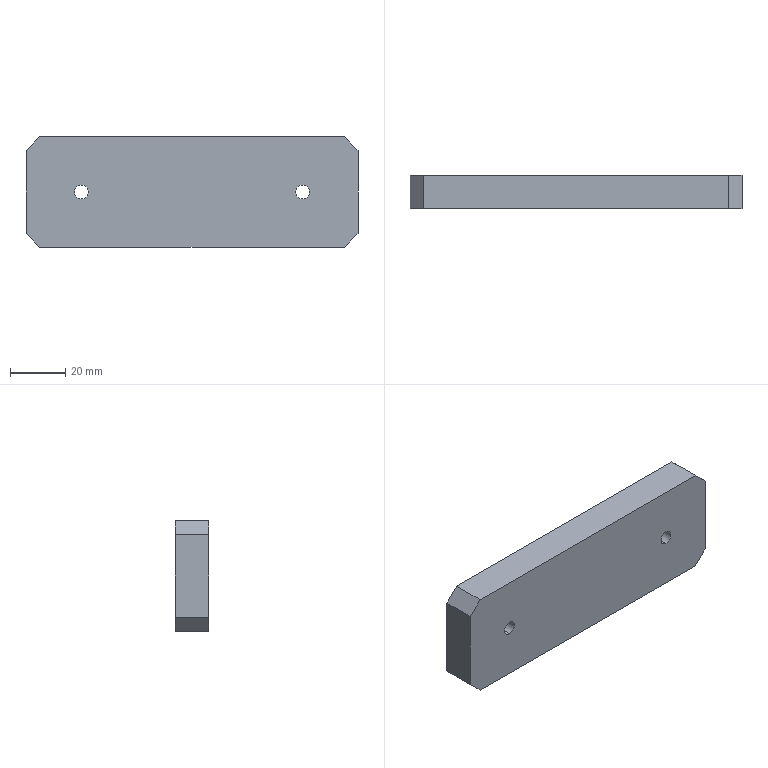Part | SolidWorks | features Chamfer 1, Extrusion 1, HoleWzd 1 | 1 solid | 14 faces | box 120 x 12 x 40 mm | volume 56529 mm3 | plane 10 | cylinder 4 | commonest cylinder face diameters 5 x4
STEP:
#1=CARTESIAN_POINT('',(-40.,-6.,-2.5));
#2=VERTEX_POINT('',#1);
#3=CARTESIAN_POINT('',(-40.,-6.,2.5));
#4=VERTEX_POINT('',#3);
#5=CARTESIAN_POINT('',(-40.,-6.,0.));
#6=DIRECTION('',(0.,1.,0.));
#7=DIRECTION('',(0.,0.,1.));
#8=AXIS2_PLACEMENT_3D('',#5,#6,#7);
#9=CIRCLE('',#8,2.5);
#10=EDGE_CURVE('',#2,#4,#9,.T.);
#11=ORIENTED_EDGE('',*,*,#10,.F.);
#12=CARTESIAN_POINT('',(-40.,6.,-2.5));
#13=VERTEX_POINT('',#12);
#14=CARTESIAN_POINT('',(-40.,6.,-2.5));
#15=DIRECTION('',(0.,1.,0.));
#16=VECTOR('',#15,1000.);
#17=LINE('',#14,#16);
#18=EDGE_CURVE('',#2,#13,#17,.T.);
#19=ORIENTED_EDGE('',*,*,#18,.T.);
#20=CARTESIAN_POINT('',(-40.,6.,2.5));
#21=VERTEX_POINT('',#20);
#22=CARTESIAN_POINT('',(-40.,6.,0.));
#23=DIRECTION('',(0.,1.,0.));
#24=DIRECTION('',(0.,0.,1.));
#25=AXIS2_PLACEMENT_3D('',#22,#23,#24);
#26=CIRCLE('',#25,2.5);
#27=EDGE_CURVE('',#13,#21,#26,.T.);
#28=ORIENTED_EDGE('',*,*,#27,.T.);
#29=CARTESIAN_POINT('',(-40.,6.,2.5));
#30=DIRECTION('',(0.,1.,0.));
#31=VECTOR('',#30,1000.);
#32=LINE('',#29,#31);
#33=EDGE_CURVE('',#4,#21,#32,.T.);
#34=ORIENTED_EDGE('',*,*,#33,.F.);
#35=EDGE_LOOP('',(#11,#19,#28,#34));
#36=FACE_OUTER_BOUND('',#35,.T.);
#37=CARTESIAN_POINT('',(-40.,6.,0.));
#38=DIRECTION('',(0.,1.,0.));
#39=DIRECTION('',(0.,0.,1.));
#40=AXIS2_PLACEMENT_3D('',#37,#38,#39);
#41=CYLINDRICAL_SURFACE('',#40,2.5);
#42=ADVANCED_FACE('',(#36),#41,.F.);
#43=CARTESIAN_POINT('',(40.,-6.,-2.5));
#44=VERTEX_POINT('',#43);
#45=CARTESIAN_POINT('',(40.,-6.,2.5));
#46=VERTEX_POINT('',#45);
#47=CARTESIAN_POINT('',(40.,-6.,0.));
#48=DIRECTION('',(0.,1.,0.));
#49=DIRECTION('',(0.,0.,1.));
#50=AXIS2_PLACEMENT_3D('',#47,#48,#49);
#51=CIRCLE('',#50,2.5);
#52=EDGE_CURVE('',#44,#46,#51,.T.);
#53=ORIENTED_EDGE('',*,*,#52,.F.);
#54=CARTESIAN_POINT('',(40.,6.,-2.5));
#55=VERTEX_POINT('',#54);
#56=CARTESIAN_POINT('',(40.,6.,-2.5));
#57=DIRECTION('',(0.,1.,0.));
#58=VECTOR('',#57,1000.);
#59=LINE('',#56,#58);
#60=EDGE_CURVE('',#44,#55,#59,.T.);
#61=ORIENTED_EDGE('',*,*,#60,.T.);
#62=CARTESIAN_POINT('',(40.,6.,2.5));
#63=VERTEX_POINT('',#62);
#64=CARTESIAN_POINT('',(40.,6.,0.));
#65=DIRECTION('',(0.,1.,0.));
#66=DIRECTION('',(0.,0.,1.));
#67=AXIS2_PLACEMENT_3D('',#64,#65,#66);
#68=CIRCLE('',#67,2.5);
#69=EDGE_CURVE('',#55,#63,#68,.T.);
#70=ORIENTED_EDGE('',*,*,#69,.T.);
#71=CARTESIAN_POINT('',(40.,6.,2.5));
#72=DIRECTION('',(0.,1.,0.));
#73=VECTOR('',#72,1000.);
#74=LINE('',#71,#73);
#75=EDGE_CURVE('',#46,#63,#74,.T.);
#76=ORIENTED_EDGE('',*,*,#75,.F.);
#77=EDGE_LOOP('',(#53,#61,#70,#76));
#78=FACE_OUTER_BOUND('',#77,.T.);
#79=CARTESIAN_POINT('',(40.,6.,0.));
#80=DIRECTION('',(0.,1.,0.));
#81=DIRECTION('',(0.,0.,1.));
#82=AXIS2_PLACEMENT_3D('',#79,#80,#81);
#83=CYLINDRICAL_SURFACE('',#82,2.5);
#84=ADVANCED_FACE('',(#78),#83,.F.);
#85=CARTESIAN_POINT('',(-60.,-6.,-15.));
#86=VERTEX_POINT('',#85);
#87=CARTESIAN_POINT('',(-60.,-6.,15.));
#88=VERTEX_POINT('',#87);
#89=CARTESIAN_POINT('',(-60.,-6.,-20.));
#90=DIRECTION('',(0.,0.,1.));
#91=VECTOR('',#90,1000.);
#92=LINE('',#89,#91);
#93=EDGE_CURVE('',#86,#88,#92,.T.);
#94=ORIENTED_EDGE('',*,*,#93,.T.);
#95=CARTESIAN_POINT('',(-60.,6.,15.));
#96=VERTEX_POINT('',#95);
#97=CARTESIAN_POINT('',(-60.,6.,15.));
#98=DIRECTION('',(0.,1.,0.));
#99=VECTOR('',#98,1000.);
#100=LINE('',#97,#99);
#101=EDGE_CURVE('',#88,#96,#100,.T.);
#102=ORIENTED_EDGE('',*,*,#101,.T.);
#103=CARTESIAN_POINT('',(-60.,6.,-15.));
#104=VERTEX_POINT('',#103);
#105=CARTESIAN_POINT('',(-60.,6.,-20.));
#106=DIRECTION('',(0.,0.,1.));
#107=VECTOR('',#106,1000.);
#108=LINE('',#105,#107);
#109=EDGE_CURVE('',#104,#96,#108,.T.);
#110=ORIENTED_EDGE('',*,*,#109,.F.);
#111=CARTESIAN_POINT('',(-60.,6.,-15.));
#112=DIRECTION('',(0.,-1.,0.));
#113=VECTOR('',#112,1000.);
#114=LINE('',#111,#113);
#115=EDGE_CURVE('',#104,#86,#114,.T.);
#116=ORIENTED_EDGE('',*,*,#115,.T.);
#117=EDGE_LOOP('',(#94,#102,#110,#116));
#118=FACE_OUTER_BOUND('',#117,.T.);
#119=CARTESIAN_POINT('',(-60.,6.,-20.));
#120=DIRECTION('',(1.,0.,0.));
#121=DIRECTION('',(0.,0.,-1.));
#122=AXIS2_PLACEMENT_3D('',#119,#120,#121);
#123=PLANE('',#122);
#124=ADVANCED_FACE('',(#118),#123,.F.);
#125=CARTESIAN_POINT('',(-55.,-6.,20.));
#126=VERTEX_POINT('',#125);
#127=CARTESIAN_POINT('',(55.,-6.,20.));
#128=VERTEX_POINT('',#127);
#129=CARTESIAN_POINT('',(-60.,-6.,20.));
#130=DIRECTION('',(1.,0.,0.));
#131=VECTOR('',#130,1000.);
#132=LINE('',#129,#131);
#133=EDGE_CURVE('',#126,#128,#132,.T.);
#134=ORIENTED_EDGE('',*,*,#133,.T.);
#135=CARTESIAN_POINT('',(55.,6.,20.));
#136=VERTEX_POINT('',#135);
#137=CARTESIAN_POINT('',(55.,6.,20.));
#138=DIRECTION('',(0.,1.,0.));
#139=VECTOR('',#138,1000.);
#140=LINE('',#137,#139);
#141=EDGE_CURVE('',#128,#136,#140,.T.);
#142=ORIENTED_EDGE('',*,*,#141,.T.);
#143=CARTESIAN_POINT('',(-55.,6.,20.));
#144=VERTEX_POINT('',#143);
#145=CARTESIAN_POINT('',(-60.,6.,20.));
#146=DIRECTION('',(1.,0.,0.));
#147=VECTOR('',#146,1000.);
#148=LINE('',#145,#147);
#149=EDGE_CURVE('',#144,#136,#148,.T.);
#150=ORIENTED_EDGE('',*,*,#149,.F.);
#151=CARTESIAN_POINT('',(-55.,6.,20.));
#152=DIRECTION('',(0.,-1.,0.));
#153=VECTOR('',#152,1000.);
#154=LINE('',#151,#153);
#155=EDGE_CURVE('',#144,#126,#154,.T.);
#156=ORIENTED_EDGE('',*,*,#155,.T.);
#157=EDGE_LOOP('',(#134,#142,#150,#156));
#158=FACE_OUTER_BOUND('',#157,.T.);
#159=CARTESIAN_POINT('',(-60.,6.,20.));
#160=DIRECTION('',(0.,0.,-1.));
#161=DIRECTION('',(-1.,0.,0.));
#162=AXIS2_PLACEMENT_3D('',#159,#160,#161);
#163=PLANE('',#162);
#164=ADVANCED_FACE('',(#158),#163,.F.);
#165=CARTESIAN_POINT('',(60.,6.,15.));
#166=VERTEX_POINT('',#165);
#167=CARTESIAN_POINT('',(60.,6.,-15.));
#168=VERTEX_POINT('',#167);
#169=CARTESIAN_POINT('',(60.,6.,-20.));
#170=DIRECTION('',(0.,0.,-1.));
#171=VECTOR('',#170,1000.);
#172=LINE('',#169,#171);
#173=EDGE_CURVE('',#166,#168,#172,.T.);
#174=ORIENTED_EDGE('',*,*,#173,.F.);
#175=CARTESIAN_POINT('',(60.,-6.,15.));
#176=VERTEX_POINT('',#175);
#177=CARTESIAN_POINT('',(60.,6.,15.));
#178=DIRECTION('',(0.,-1.,0.));
#179=VECTOR('',#178,1000.);
#180=LINE('',#177,#179);
#181=EDGE_CURVE('',#166,#176,#180,.T.);
#182=ORIENTED_EDGE('',*,*,#181,.T.);
#183=CARTESIAN_POINT('',(60.,-6.,-15.));
#184=VERTEX_POINT('',#183);
#185=CARTESIAN_POINT('',(60.,-6.,-20.));
#186=DIRECTION('',(0.,0.,-1.));
#187=VECTOR('',#186,1000.);
#188=LINE('',#185,#187);
#189=EDGE_CURVE('',#176,#184,#188,.T.);
#190=ORIENTED_EDGE('',*,*,#189,.T.);
#191=CARTESIAN_POINT('',(60.,6.,-15.));
#192=DIRECTION('',(0.,1.,0.));
#193=VECTOR('',#192,1000.);
#194=LINE('',#191,#193);
#195=EDGE_CURVE('',#184,#168,#194,.T.);
#196=ORIENTED_EDGE('',*,*,#195,.T.);
#197=EDGE_LOOP('',(#174,#182,#190,#196));
#198=FACE_OUTER_BOUND('',#197,.T.);
#199=CARTESIAN_POINT('',(60.,6.,-20.));
#200=DIRECTION('',(-1.,0.,0.));
#201=DIRECTION('',(0.,0.,1.));
#202=AXIS2_PLACEMENT_3D('',#199,#200,#201);
#203=PLANE('',#202);
#204=ADVANCED_FACE('',(#198),#203,.F.);
#205=CARTESIAN_POINT('',(55.,-6.,-20.));
#206=VERTEX_POINT('',#205);
#207=CARTESIAN_POINT('',(-55.,-6.,-20.));
#208=VERTEX_POINT('',#207);
#209=CARTESIAN_POINT('',(-60.,-6.,-20.));
#210=DIRECTION('',(-1.,0.,0.));
#211=VECTOR('',#210,1000.);
#212=LINE('',#209,#211);
#213=EDGE_CURVE('',#206,#208,#212,.T.);
#214=ORIENTED_EDGE('',*,*,#213,.T.);
#215=CARTESIAN_POINT('',(-55.,6.,-20.));
#216=VERTEX_POINT('',#215);
#217=CARTESIAN_POINT('',(-55.,6.,-20.));
#218=DIRECTION('',(0.,1.,0.));
#219=VECTOR('',#218,1000.);
#220=LINE('',#217,#219);
#221=EDGE_CURVE('',#208,#216,#220,.T.);
#222=ORIENTED_EDGE('',*,*,#221,.T.);
#223=CARTESIAN_POINT('',(55.,6.,-20.));
#224=VERTEX_POINT('',#223);
#225=CARTESIAN_POINT('',(-60.,6.,-20.));
#226=DIRECTION('',(-1.,0.,0.));
#227=VECTOR('',#226,1000.);
#228=LINE('',#225,#227);
#229=EDGE_CURVE('',#224,#216,#228,.T.);
#230=ORIENTED_EDGE('',*,*,#229,.F.);
#231=CARTESIAN_POINT('',(55.,6.,-20.));
#232=DIRECTION('',(0.,-1.,0.));
#233=VECTOR('',#232,1000.);
#234=LINE('',#231,#233);
#235=EDGE_CURVE('',#224,#206,#234,.T.);
#236=ORIENTED_EDGE('',*,*,#235,.T.);
#237=EDGE_LOOP('',(#214,#222,#230,#236));
#238=FACE_OUTER_BOUND('',#237,.T.);
#239=CARTESIAN_POINT('',(-60.,6.,-20.));
#240=DIRECTION('',(0.,0.,1.));
#241=DIRECTION('',(1.,0.,0.));
#242=AXIS2_PLACEMENT_3D('',#239,#240,#241);
#243=PLANE('',#242);
#244=ADVANCED_FACE('',(#238),#243,.F.);
#245=CARTESIAN_POINT('',(-40.,6.,0.));
#246=DIRECTION('',(0.,1.,0.));
#247=DIRECTION('',(0.,0.,1.));
#248=AXIS2_PLACEMENT_3D('',#245,#246,#247);
#249=CIRCLE('',#248,2.5);
#250=EDGE_CURVE('',#21,#13,#249,.T.);
#251=ORIENTED_EDGE('',*,*,#250,.F.);
#252=ORIENTED_EDGE('',*,*,#27,.F.);
#253=EDGE_LOOP('',(#251,#252));
#254=FACE_BOUND('',#253,.T.);
#255=CARTESIAN_POINT('',(40.,6.,0.));
#256=DIRECTION('',(0.,1.,0.));
#257=DIRECTION('',(0.,0.,1.));
#258=AXIS2_PLACEMENT_3D('',#255,#256,#257);
#259=CIRCLE('',#258,2.5);
#260=EDGE_CURVE('',#63,#55,#259,.T.);
#261=ORIENTED_EDGE('',*,*,#260,.F.);
#262=ORIENTED_EDGE('',*,*,#69,.F.);
#263=EDGE_LOOP('',(#261,#262));
#264=FACE_BOUND('',#263,.T.);
#265=ORIENTED_EDGE('',*,*,#149,.T.);
#266=CARTESIAN_POINT('',(-2.5,6.,77.5));
#267=DIRECTION('',(0.7071,0.,-0.7071));
#268=VECTOR('',#267,1000.);
#269=LINE('',#266,#268);
#270=EDGE_CURVE('',#136,#166,#269,.T.);
#271=ORIENTED_EDGE('',*,*,#270,.T.);
#272=ORIENTED_EDGE('',*,*,#173,.T.);
#273=CARTESIAN_POINT('',(17.5,6.,-57.5));
#274=DIRECTION('',(-0.7071,0.,-0.7071));
#275=VECTOR('',#274,1000.);
#276=LINE('',#273,#275);
#277=EDGE_CURVE('',#168,#224,#276,.T.);
#278=ORIENTED_EDGE('',*,*,#277,.T.);
#279=ORIENTED_EDGE('',*,*,#229,.T.);
#280=CARTESIAN_POINT('',(-77.5,6.,2.5));
#281=DIRECTION('',(-0.7071,0.,0.7071));
#282=VECTOR('',#281,1000.);
#283=LINE('',#280,#282);
#284=EDGE_CURVE('',#216,#104,#283,.T.);
#285=ORIENTED_EDGE('',*,*,#284,.T.);
#286=ORIENTED_EDGE('',*,*,#109,.T.);
#287=CARTESIAN_POINT('',(-57.5,6.,17.5));
#288=DIRECTION('',(0.7071,0.,0.7071));
#289=VECTOR('',#288,1000.);
#290=LINE('',#287,#289);
#291=EDGE_CURVE('',#96,#144,#290,.T.);
#292=ORIENTED_EDGE('',*,*,#291,.T.);
#293=EDGE_LOOP('',(#265,#271,#272,#278,#279,#285,#286,#292));
#294=FACE_OUTER_BOUND('',#293,.T.);
#295=CARTESIAN_POINT('',(-60.,6.,20.));
#296=DIRECTION('',(0.,1.,0.));
#297=DIRECTION('',(0.,0.,1.));
#298=AXIS2_PLACEMENT_3D('',#295,#296,#297);
#299=PLANE('',#298);
#300=ADVANCED_FACE('',(#254,#264,#294),#299,.T.);
#301=CARTESIAN_POINT('',(-40.,-6.,0.));
#302=DIRECTION('',(0.,1.,0.));
#303=DIRECTION('',(0.,0.,1.));
#304=AXIS2_PLACEMENT_3D('',#301,#302,#303);
#305=CIRCLE('',#304,2.5);
#306=EDGE_CURVE('',#4,#2,#305,.T.);
#307=ORIENTED_EDGE('',*,*,#306,.T.);
#308=ORIENTED_EDGE('',*,*,#10,.T.);
#309=EDGE_LOOP('',(#307,#308));
#310=FACE_BOUND('',#309,.T.);
#311=CARTESIAN_POINT('',(40.,-6.,0.));
#312=DIRECTION('',(0.,1.,0.));
#313=DIRECTION('',(0.,0.,1.));
#314=AXIS2_PLACEMENT_3D('',#311,#312,#313);
#315=CIRCLE('',#314,2.5);
#316=EDGE_CURVE('',#46,#44,#315,.T.);
#317=ORIENTED_EDGE('',*,*,#316,.T.);
#318=ORIENTED_EDGE('',*,*,#52,.T.);
#319=EDGE_LOOP('',(#317,#318));
#320=FACE_BOUND('',#319,.T.);
#321=ORIENTED_EDGE('',*,*,#189,.F.);
#322=CARTESIAN_POINT('',(60.,-6.,15.));
#323=DIRECTION('',(-0.7071,0.,0.7071));
#324=VECTOR('',#323,1000.);
#325=LINE('',#322,#324);
#326=EDGE_CURVE('',#176,#128,#325,.T.);
#327=ORIENTED_EDGE('',*,*,#326,.T.);
#328=ORIENTED_EDGE('',*,*,#133,.F.);
#329=CARTESIAN_POINT('',(-55.,-6.,20.));
#330=DIRECTION('',(-0.7071,0.,-0.7071));
#331=VECTOR('',#330,1000.);
#332=LINE('',#329,#331);
#333=EDGE_CURVE('',#126,#88,#332,.T.);
#334=ORIENTED_EDGE('',*,*,#333,.T.);
#335=ORIENTED_EDGE('',*,*,#93,.F.);
#336=CARTESIAN_POINT('',(-60.,-6.,-15.));
#337=DIRECTION('',(0.7071,0.,-0.7071));
#338=VECTOR('',#337,1000.);
#339=LINE('',#336,#338);
#340=EDGE_CURVE('',#86,#208,#339,.T.);
#341=ORIENTED_EDGE('',*,*,#340,.T.);
#342=ORIENTED_EDGE('',*,*,#213,.F.);
#343=CARTESIAN_POINT('',(55.,-6.,-20.));
#344=DIRECTION('',(0.7071,0.,0.7071));
#345=VECTOR('',#344,1000.);
#346=LINE('',#343,#345);
#347=EDGE_CURVE('',#206,#184,#346,.T.);
#348=ORIENTED_EDGE('',*,*,#347,.T.);
#349=EDGE_LOOP('',(#321,#327,#328,#334,#335,#341,#342,#348));
#350=FACE_OUTER_BOUND('',#349,.T.);
#351=CARTESIAN_POINT('',(-60.,-6.,20.));
#352=DIRECTION('',(0.,1.,0.));
#353=DIRECTION('',(0.,0.,1.));
#354=AXIS2_PLACEMENT_3D('',#351,#352,#353);
#355=PLANE('',#354);
#356=ADVANCED_FACE('',(#310,#320,#350),#355,.F.);
#357=ORIENTED_EDGE('',*,*,#60,.F.);
#358=ORIENTED_EDGE('',*,*,#316,.F.);
#359=ORIENTED_EDGE('',*,*,#75,.T.);
#360=ORIENTED_EDGE('',*,*,#260,.T.);
#361=EDGE_LOOP('',(#357,#358,#359,#360));
#362=FACE_OUTER_BOUND('',#361,.T.);
#363=CARTESIAN_POINT('',(40.,6.,0.));
#364=DIRECTION('',(0.,1.,0.));
#365=DIRECTION('',(0.,0.,1.));
#366=AXIS2_PLACEMENT_3D('',#363,#364,#365);
#367=CYLINDRICAL_SURFACE('',#366,2.5);
#368=ADVANCED_FACE('',(#362),#367,.F.);
#369=ORIENTED_EDGE('',*,*,#18,.F.);
#370=ORIENTED_EDGE('',*,*,#306,.F.);
#371=ORIENTED_EDGE('',*,*,#33,.T.);
#372=ORIENTED_EDGE('',*,*,#250,.T.);
#373=EDGE_LOOP('',(#369,#370,#371,#372));
#374=FACE_OUTER_BOUND('',#373,.T.);
#375=CARTESIAN_POINT('',(-40.,6.,0.));
#376=DIRECTION('',(0.,1.,0.));
#377=DIRECTION('',(0.,0.,1.));
#378=AXIS2_PLACEMENT_3D('',#375,#376,#377);
#379=CYLINDRICAL_SURFACE('',#378,2.5);
#380=ADVANCED_FACE('',(#374),#379,.F.);
#381=ORIENTED_EDGE('',*,*,#270,.F.);
#382=ORIENTED_EDGE('',*,*,#141,.F.);
#383=ORIENTED_EDGE('',*,*,#326,.F.);
#384=ORIENTED_EDGE('',*,*,#181,.F.);
#385=EDGE_LOOP('',(#381,#382,#383,#384));
#386=FACE_OUTER_BOUND('',#385,.T.);
#387=CARTESIAN_POINT('',(60.,6.,15.));
#388=DIRECTION('',(-0.7071,0.,-0.7071));
#389=DIRECTION('',(-0.7071,0.,0.7071));
#390=AXIS2_PLACEMENT_3D('',#387,#388,#389);
#391=PLANE('',#390);
#392=ADVANCED_FACE('',(#386),#391,.F.);
#393=ORIENTED_EDGE('',*,*,#291,.F.);
#394=ORIENTED_EDGE('',*,*,#101,.F.);
#395=ORIENTED_EDGE('',*,*,#333,.F.);
#396=ORIENTED_EDGE('',*,*,#155,.F.);
#397=EDGE_LOOP('',(#393,#394,#395,#396));
#398=FACE_OUTER_BOUND('',#397,.T.);
#399=CARTESIAN_POINT('',(-55.,6.,20.));
#400=DIRECTION('',(0.7071,0.,-0.7071));
#401=DIRECTION('',(-0.7071,0.,-0.7071));
#402=AXIS2_PLACEMENT_3D('',#399,#400,#401);
#403=PLANE('',#402);
#404=ADVANCED_FACE('',(#398),#403,.F.);
#405=ORIENTED_EDGE('',*,*,#284,.F.);
#406=ORIENTED_EDGE('',*,*,#221,.F.);
#407=ORIENTED_EDGE('',*,*,#340,.F.);
#408=ORIENTED_EDGE('',*,*,#115,.F.);
#409=EDGE_LOOP('',(#405,#406,#407,#408));
#410=FACE_OUTER_BOUND('',#409,.T.);
#411=CARTESIAN_POINT('',(-60.,6.,-15.));
#412=DIRECTION('',(0.7071,0.,0.7071));
#413=DIRECTION('',(0.7071,0.,-0.7071));
#414=AXIS2_PLACEMENT_3D('',#411,#412,#413);
#415=PLANE('',#414);
#416=ADVANCED_FACE('',(#410),#415,.F.);
#417=ORIENTED_EDGE('',*,*,#277,.F.);
#418=ORIENTED_EDGE('',*,*,#195,.F.);
#419=ORIENTED_EDGE('',*,*,#347,.F.);
#420=ORIENTED_EDGE('',*,*,#235,.F.);
#421=EDGE_LOOP('',(#417,#418,#419,#420));
#422=FACE_OUTER_BOUND('',#421,.T.);
#423=CARTESIAN_POINT('',(55.,6.,-20.));
#424=DIRECTION('',(-0.7071,0.,0.7071));
#425=DIRECTION('',(0.7071,0.,0.7071));
#426=AXIS2_PLACEMENT_3D('',#423,#424,#425);
#427=PLANE('',#426);
#428=ADVANCED_FACE('',(#422),#427,.F.);
#429=CLOSED_SHELL('',(#42,#84,#124,#164,#204,#244,#300,#356,#368,#380,#392,#404,#416,#428));
#430=MANIFOLD_SOLID_BREP('',#429);
#431=CARTESIAN_POINT('',(0.,0.,0.));
#432=DIRECTION('',(0.,0.,1.));
#433=DIRECTION('',(1.,0.,0.));
#434=AXIS2_PLACEMENT_3D('',#431,#432,#433);
#435=(LENGTH_UNIT()NAMED_UNIT(*)SI_UNIT(.MILLI.,.METRE.));
#436=UNCERTAINTY_MEASURE_WITH_UNIT(LENGTH_MEASURE(0.00001),#435,'','');
#437=(NAMED_UNIT(*)PLANE_ANGLE_UNIT()SI_UNIT($,.RADIAN.));
#438=(NAMED_UNIT(*)SI_UNIT($,.STERADIAN.)SOLID_ANGLE_UNIT());
#439=(GEOMETRIC_REPRESENTATION_CONTEXT(3)GLOBAL_UNCERTAINTY_ASSIGNED_CONTEXT((#436))GLOBAL_UNIT_ASSIGNED_CONTEXT((#435,#437,#438))REPRESENTATION_CONTEXT('',''));
#440=ADVANCED_BREP_SHAPE_REPRESENTATION('',(#430,#434),#439);